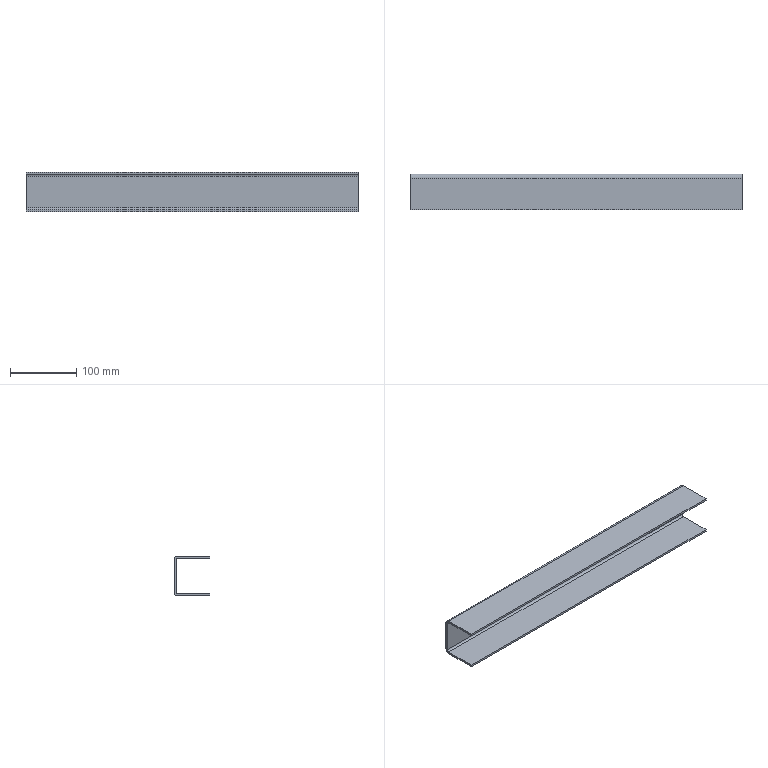Part | STEP file | JBJ-P-1015-02_Default<As Machined> | 1 solid | 22 faces | box 500 x 54 x 60 mm | volume 237206 mm3 | plane 18 | cylinder 4 | commonest cylinder face diameters 6 x2 12 x2
STEP:
#1=CARTESIAN_POINT('',(500.,54.,-6.));
#2=VERTEX_POINT('',#1);
#3=CARTESIAN_POINT('',(500.,51.,-6.));
#4=VERTEX_POINT('',#3);
#5=CARTESIAN_POINT('',(500.,54.,-6.));
#6=DIRECTION('',(0.,-1.,0.));
#7=VECTOR('',#6,1000.);
#8=LINE('',#5,#7);
#9=EDGE_CURVE('',#2,#4,#8,.T.);
#10=ORIENTED_EDGE('',*,*,#9,.F.);
#11=CARTESIAN_POINT('',(500.,48.,0.));
#12=VERTEX_POINT('',#11);
#13=CARTESIAN_POINT('',(500.,48.,-6.));
#14=DIRECTION('',(-1.,0.,0.));
#15=DIRECTION('',(0.,0.,-1.));
#16=AXIS2_PLACEMENT_3D('',#13,#14,#15);
#17=CIRCLE('',#16,6.);
#18=EDGE_CURVE('',#12,#2,#17,.T.);
#19=ORIENTED_EDGE('',*,*,#18,.F.);
#20=CARTESIAN_POINT('',(500.,48.,-3.));
#21=VERTEX_POINT('',#20);
#22=CARTESIAN_POINT('',(500.,48.,-3.));
#23=DIRECTION('',(0.,0.,1.));
#24=VECTOR('',#23,1000.);
#25=LINE('',#22,#24);
#26=EDGE_CURVE('',#21,#12,#25,.T.);
#27=ORIENTED_EDGE('',*,*,#26,.F.);
#28=CARTESIAN_POINT('',(500.,48.,-6.));
#29=DIRECTION('',(-1.,0.,0.));
#30=DIRECTION('',(0.,0.,-1.));
#31=AXIS2_PLACEMENT_3D('',#28,#29,#30);
#32=CIRCLE('',#31,3.);
#33=EDGE_CURVE('',#21,#4,#32,.T.);
#34=ORIENTED_EDGE('',*,*,#33,.T.);
#35=EDGE_LOOP('',(#10,#19,#27,#34));
#36=FACE_OUTER_BOUND('',#35,.T.);
#37=CARTESIAN_POINT('',(500.,54.,-6.));
#38=DIRECTION('',(1.,0.,0.));
#39=DIRECTION('',(0.,0.,-1.));
#40=AXIS2_PLACEMENT_3D('',#37,#38,#39);
#41=PLANE('',#40);
#42=ADVANCED_FACE('',(#36),#41,.T.);
#43=CARTESIAN_POINT('',(500.,54.,-54.));
#44=VERTEX_POINT('',#43);
#45=CARTESIAN_POINT('',(500.,54.,0.));
#46=DIRECTION('',(0.,0.,-1.));
#47=VECTOR('',#46,1000.);
#48=LINE('',#45,#47);
#49=EDGE_CURVE('',#2,#44,#48,.T.);
#50=ORIENTED_EDGE('',*,*,#49,.F.);
#51=ORIENTED_EDGE('',*,*,#9,.T.);
#52=CARTESIAN_POINT('',(500.,51.,-54.));
#53=VERTEX_POINT('',#52);
#54=CARTESIAN_POINT('',(500.,51.,0.));
#55=DIRECTION('',(0.,0.,-1.));
#56=VECTOR('',#55,1000.);
#57=LINE('',#54,#56);
#58=EDGE_CURVE('',#4,#53,#57,.T.);
#59=ORIENTED_EDGE('',*,*,#58,.T.);
#60=CARTESIAN_POINT('',(500.,51.,-54.));
#61=DIRECTION('',(0.,1.,0.));
#62=VECTOR('',#61,1000.);
#63=LINE('',#60,#62);
#64=EDGE_CURVE('',#53,#44,#63,.T.);
#65=ORIENTED_EDGE('',*,*,#64,.T.);
#66=EDGE_LOOP('',(#50,#51,#59,#65));
#67=FACE_OUTER_BOUND('',#66,.T.);
#68=CARTESIAN_POINT('',(500.,48.,-3.));
#69=DIRECTION('',(1.,0.,0.));
#70=DIRECTION('',(0.,0.,-1.));
#71=AXIS2_PLACEMENT_3D('',#68,#69,#70);
#72=PLANE('',#71);
#73=ADVANCED_FACE('',(#67),#72,.T.);
#74=CARTESIAN_POINT('',(0.,48.,0.));
#75=VERTEX_POINT('',#74);
#76=CARTESIAN_POINT('',(0.,48.,-3.));
#77=VERTEX_POINT('',#76);
#78=CARTESIAN_POINT('',(0.,48.,0.));
#79=DIRECTION('',(0.,0.,-1.));
#80=VECTOR('',#79,1000.);
#81=LINE('',#78,#80);
#82=EDGE_CURVE('',#75,#77,#81,.T.);
#83=ORIENTED_EDGE('',*,*,#82,.F.);
#84=CARTESIAN_POINT('',(0.,54.,-6.));
#85=VERTEX_POINT('',#84);
#86=CARTESIAN_POINT('',(0.,48.,-6.));
#87=DIRECTION('',(-1.,0.,0.));
#88=DIRECTION('',(0.,0.,-1.));
#89=AXIS2_PLACEMENT_3D('',#86,#87,#88);
#90=CIRCLE('',#89,6.);
#91=EDGE_CURVE('',#75,#85,#90,.T.);
#92=ORIENTED_EDGE('',*,*,#91,.T.);
#93=CARTESIAN_POINT('',(0.,51.,-6.));
#94=VERTEX_POINT('',#93);
#95=CARTESIAN_POINT('',(0.,51.,-6.));
#96=DIRECTION('',(0.,1.,0.));
#97=VECTOR('',#96,1000.);
#98=LINE('',#95,#97);
#99=EDGE_CURVE('',#94,#85,#98,.T.);
#100=ORIENTED_EDGE('',*,*,#99,.F.);
#101=CARTESIAN_POINT('',(0.,48.,-6.));
#102=DIRECTION('',(-1.,0.,0.));
#103=DIRECTION('',(0.,0.,-1.));
#104=AXIS2_PLACEMENT_3D('',#101,#102,#103);
#105=CIRCLE('',#104,3.);
#106=EDGE_CURVE('',#77,#94,#105,.T.);
#107=ORIENTED_EDGE('',*,*,#106,.F.);
#108=EDGE_LOOP('',(#83,#92,#100,#107));
#109=FACE_OUTER_BOUND('',#108,.T.);
#110=CARTESIAN_POINT('',(0.,48.,0.));
#111=DIRECTION('',(-1.,0.,0.));
#112=DIRECTION('',(0.,0.,1.));
#113=AXIS2_PLACEMENT_3D('',#110,#111,#112);
#114=PLANE('',#113);
#115=ADVANCED_FACE('',(#109),#114,.T.);
#116=CARTESIAN_POINT('',(0.,0.,0.));
#117=VERTEX_POINT('',#116);
#118=CARTESIAN_POINT('',(0.,0.,0.));
#119=DIRECTION('',(0.,1.,0.));
#120=VECTOR('',#119,1000.);
#121=LINE('',#118,#120);
#122=EDGE_CURVE('',#117,#75,#121,.T.);
#123=ORIENTED_EDGE('',*,*,#122,.T.);
#124=ORIENTED_EDGE('',*,*,#82,.T.);
#125=CARTESIAN_POINT('',(0.,0.,-3.));
#126=VERTEX_POINT('',#125);
#127=CARTESIAN_POINT('',(0.,0.,-3.));
#128=DIRECTION('',(0.,1.,0.));
#129=VECTOR('',#128,1000.);
#130=LINE('',#127,#129);
#131=EDGE_CURVE('',#126,#77,#130,.T.);
#132=ORIENTED_EDGE('',*,*,#131,.F.);
#133=CARTESIAN_POINT('',(0.,0.,-3.));
#134=DIRECTION('',(0.,0.,1.));
#135=VECTOR('',#134,1000.);
#136=LINE('',#133,#135);
#137=EDGE_CURVE('',#126,#117,#136,.T.);
#138=ORIENTED_EDGE('',*,*,#137,.T.);
#139=EDGE_LOOP('',(#123,#124,#132,#138));
#140=FACE_OUTER_BOUND('',#139,.T.);
#141=CARTESIAN_POINT('',(0.,51.,-6.));
#142=DIRECTION('',(-1.,0.,0.));
#143=DIRECTION('',(0.,0.,1.));
#144=AXIS2_PLACEMENT_3D('',#141,#142,#143);
#145=PLANE('',#144);
#146=ADVANCED_FACE('',(#140),#145,.T.);
#147=CARTESIAN_POINT('',(500.,48.,-60.));
#148=VERTEX_POINT('',#147);
#149=CARTESIAN_POINT('',(500.,48.,-57.));
#150=VERTEX_POINT('',#149);
#151=CARTESIAN_POINT('',(500.,48.,-60.));
#152=DIRECTION('',(0.,0.,1.));
#153=VECTOR('',#152,1000.);
#154=LINE('',#151,#153);
#155=EDGE_CURVE('',#148,#150,#154,.T.);
#156=ORIENTED_EDGE('',*,*,#155,.F.);
#157=CARTESIAN_POINT('',(500.,48.,-54.));
#158=DIRECTION('',(-1.,0.,0.));
#159=DIRECTION('',(0.,0.,-1.));
#160=AXIS2_PLACEMENT_3D('',#157,#158,#159);
#161=CIRCLE('',#160,6.);
#162=EDGE_CURVE('',#44,#148,#161,.T.);
#163=ORIENTED_EDGE('',*,*,#162,.F.);
#164=ORIENTED_EDGE('',*,*,#64,.F.);
#165=CARTESIAN_POINT('',(500.,48.,-54.));
#166=DIRECTION('',(-1.,0.,0.));
#167=DIRECTION('',(0.,0.,-1.));
#168=AXIS2_PLACEMENT_3D('',#165,#166,#167);
#169=CIRCLE('',#168,3.);
#170=EDGE_CURVE('',#53,#150,#169,.T.);
#171=ORIENTED_EDGE('',*,*,#170,.T.);
#172=EDGE_LOOP('',(#156,#163,#164,#171));
#173=FACE_OUTER_BOUND('',#172,.T.);
#174=CARTESIAN_POINT('',(500.,48.,-60.));
#175=DIRECTION('',(1.,0.,0.));
#176=DIRECTION('',(0.,0.,-1.));
#177=AXIS2_PLACEMENT_3D('',#174,#175,#176);
#178=PLANE('',#177);
#179=ADVANCED_FACE('',(#173),#178,.T.);
#180=CARTESIAN_POINT('',(500.,0.,-60.));
#181=VERTEX_POINT('',#180);
#182=CARTESIAN_POINT('',(500.,54.,-60.));
#183=DIRECTION('',(0.,-1.,0.));
#184=VECTOR('',#183,1000.);
#185=LINE('',#182,#184);
#186=EDGE_CURVE('',#148,#181,#185,.T.);
#187=ORIENTED_EDGE('',*,*,#186,.F.);
#188=ORIENTED_EDGE('',*,*,#155,.T.);
#189=CARTESIAN_POINT('',(500.,0.,-57.));
#190=VERTEX_POINT('',#189);
#191=CARTESIAN_POINT('',(500.,54.,-57.));
#192=DIRECTION('',(0.,-1.,0.));
#193=VECTOR('',#192,1000.);
#194=LINE('',#191,#193);
#195=EDGE_CURVE('',#150,#190,#194,.T.);
#196=ORIENTED_EDGE('',*,*,#195,.T.);
#197=CARTESIAN_POINT('',(500.,0.,-60.));
#198=DIRECTION('',(0.,0.,1.));
#199=VECTOR('',#198,1000.);
#200=LINE('',#197,#199);
#201=EDGE_CURVE('',#181,#190,#200,.T.);
#202=ORIENTED_EDGE('',*,*,#201,.F.);
#203=EDGE_LOOP('',(#187,#188,#196,#202));
#204=FACE_OUTER_BOUND('',#203,.T.);
#205=CARTESIAN_POINT('',(500.,51.,-54.));
#206=DIRECTION('',(1.,0.,0.));
#207=DIRECTION('',(0.,0.,-1.));
#208=AXIS2_PLACEMENT_3D('',#205,#206,#207);
#209=PLANE('',#208);
#210=ADVANCED_FACE('',(#204),#209,.T.);
#211=CARTESIAN_POINT('',(0.,54.,-54.));
#212=VERTEX_POINT('',#211);
#213=CARTESIAN_POINT('',(0.,51.,-54.));
#214=VERTEX_POINT('',#213);
#215=CARTESIAN_POINT('',(0.,54.,-54.));
#216=DIRECTION('',(0.,-1.,0.));
#217=VECTOR('',#216,1000.);
#218=LINE('',#215,#217);
#219=EDGE_CURVE('',#212,#214,#218,.T.);
#220=ORIENTED_EDGE('',*,*,#219,.F.);
#221=CARTESIAN_POINT('',(0.,48.,-60.));
#222=VERTEX_POINT('',#221);
#223=CARTESIAN_POINT('',(0.,48.,-54.));
#224=DIRECTION('',(-1.,0.,0.));
#225=DIRECTION('',(0.,0.,-1.));
#226=AXIS2_PLACEMENT_3D('',#223,#224,#225);
#227=CIRCLE('',#226,6.);
#228=EDGE_CURVE('',#212,#222,#227,.T.);
#229=ORIENTED_EDGE('',*,*,#228,.T.);
#230=CARTESIAN_POINT('',(0.,48.,-57.));
#231=VERTEX_POINT('',#230);
#232=CARTESIAN_POINT('',(0.,48.,-57.));
#233=DIRECTION('',(0.,0.,-1.));
#234=VECTOR('',#233,1000.);
#235=LINE('',#232,#234);
#236=EDGE_CURVE('',#231,#222,#235,.T.);
#237=ORIENTED_EDGE('',*,*,#236,.F.);
#238=CARTESIAN_POINT('',(0.,48.,-54.));
#239=DIRECTION('',(-1.,0.,0.));
#240=DIRECTION('',(0.,0.,-1.));
#241=AXIS2_PLACEMENT_3D('',#238,#239,#240);
#242=CIRCLE('',#241,3.);
#243=EDGE_CURVE('',#214,#231,#242,.T.);
#244=ORIENTED_EDGE('',*,*,#243,.F.);
#245=EDGE_LOOP('',(#220,#229,#237,#244));
#246=FACE_OUTER_BOUND('',#245,.T.);
#247=CARTESIAN_POINT('',(0.,54.,-54.));
#248=DIRECTION('',(-1.,0.,0.));
#249=DIRECTION('',(0.,0.,1.));
#250=AXIS2_PLACEMENT_3D('',#247,#248,#249);
#251=PLANE('',#250);
#252=ADVANCED_FACE('',(#246),#251,.T.);
#253=CARTESIAN_POINT('',(0.,54.,0.));
#254=DIRECTION('',(0.,0.,-1.));
#255=VECTOR('',#254,1000.);
#256=LINE('',#253,#255);
#257=EDGE_CURVE('',#85,#212,#256,.T.);
#258=ORIENTED_EDGE('',*,*,#257,.T.);
#259=ORIENTED_EDGE('',*,*,#219,.T.);
#260=CARTESIAN_POINT('',(0.,51.,0.));
#261=DIRECTION('',(0.,0.,-1.));
#262=VECTOR('',#261,1000.);
#263=LINE('',#260,#262);
#264=EDGE_CURVE('',#94,#214,#263,.T.);
#265=ORIENTED_EDGE('',*,*,#264,.F.);
#266=ORIENTED_EDGE('',*,*,#99,.T.);
#267=EDGE_LOOP('',(#258,#259,#265,#266));
#268=FACE_OUTER_BOUND('',#267,.T.);
#269=CARTESIAN_POINT('',(0.,48.,-57.));
#270=DIRECTION('',(-1.,0.,0.));
#271=DIRECTION('',(0.,0.,1.));
#272=AXIS2_PLACEMENT_3D('',#269,#270,#271);
#273=PLANE('',#272);
#274=ADVANCED_FACE('',(#268),#273,.T.);
#275=CARTESIAN_POINT('',(0.,0.,-57.));
#276=VERTEX_POINT('',#275);
#277=CARTESIAN_POINT('',(0.,54.,-57.));
#278=DIRECTION('',(0.,-1.,0.));
#279=VECTOR('',#278,1000.);
#280=LINE('',#277,#279);
#281=EDGE_CURVE('',#231,#276,#280,.T.);
#282=ORIENTED_EDGE('',*,*,#281,.T.);
#283=CARTESIAN_POINT('',(500.,0.,-57.));
#284=DIRECTION('',(-1.,0.,0.));
#285=VECTOR('',#284,1000.);
#286=LINE('',#283,#285);
#287=EDGE_CURVE('',#190,#276,#286,.T.);
#288=ORIENTED_EDGE('',*,*,#287,.F.);
#289=ORIENTED_EDGE('',*,*,#195,.F.);
#290=CARTESIAN_POINT('',(500.,48.,-57.));
#291=DIRECTION('',(-1.,0.,0.));
#292=VECTOR('',#291,1000.);
#293=LINE('',#290,#292);
#294=EDGE_CURVE('',#150,#231,#293,.T.);
#295=ORIENTED_EDGE('',*,*,#294,.T.);
#296=EDGE_LOOP('',(#282,#288,#289,#295));
#297=FACE_OUTER_BOUND('',#296,.T.);
#298=CARTESIAN_POINT('',(500.,54.,-57.));
#299=DIRECTION('',(0.,0.,-1.));
#300=DIRECTION('',(-1.,0.,0.));
#301=AXIS2_PLACEMENT_3D('',#298,#299,#300);
#302=PLANE('',#301);
#303=ADVANCED_FACE('',(#297),#302,.F.);
#304=CARTESIAN_POINT('',(0.,0.,-60.));
#305=VERTEX_POINT('',#304);
#306=CARTESIAN_POINT('',(0.,0.,-60.));
#307=DIRECTION('',(0.,0.,1.));
#308=VECTOR('',#307,1000.);
#309=LINE('',#306,#308);
#310=EDGE_CURVE('',#305,#276,#309,.T.);
#311=ORIENTED_EDGE('',*,*,#310,.F.);
#312=CARTESIAN_POINT('',(500.,0.,-60.));
#313=DIRECTION('',(-1.,0.,0.));
#314=VECTOR('',#313,1000.);
#315=LINE('',#312,#314);
#316=EDGE_CURVE('',#181,#305,#315,.T.);
#317=ORIENTED_EDGE('',*,*,#316,.F.);
#318=ORIENTED_EDGE('',*,*,#201,.T.);
#319=ORIENTED_EDGE('',*,*,#287,.T.);
#320=EDGE_LOOP('',(#311,#317,#318,#319));
#321=FACE_OUTER_BOUND('',#320,.T.);
#322=CARTESIAN_POINT('',(500.,0.,-60.));
#323=DIRECTION('',(0.,-1.,0.));
#324=DIRECTION('',(0.,0.,-1.));
#325=AXIS2_PLACEMENT_3D('',#322,#323,#324);
#326=PLANE('',#325);
#327=ADVANCED_FACE('',(#321),#326,.T.);
#328=CARTESIAN_POINT('',(0.,54.,-60.));
#329=DIRECTION('',(0.,-1.,0.));
#330=VECTOR('',#329,1000.);
#331=LINE('',#328,#330);
#332=EDGE_CURVE('',#222,#305,#331,.T.);
#333=ORIENTED_EDGE('',*,*,#332,.F.);
#334=CARTESIAN_POINT('',(500.,48.,-60.));
#335=DIRECTION('',(-1.,0.,0.));
#336=VECTOR('',#335,1000.);
#337=LINE('',#334,#336);
#338=EDGE_CURVE('',#148,#222,#337,.T.);
#339=ORIENTED_EDGE('',*,*,#338,.F.);
#340=ORIENTED_EDGE('',*,*,#186,.T.);
#341=ORIENTED_EDGE('',*,*,#316,.T.);
#342=EDGE_LOOP('',(#333,#339,#340,#341));
#343=FACE_OUTER_BOUND('',#342,.T.);
#344=CARTESIAN_POINT('',(500.,54.,-60.));
#345=DIRECTION('',(0.,0.,-1.));
#346=DIRECTION('',(-1.,0.,0.));
#347=AXIS2_PLACEMENT_3D('',#344,#345,#346);
#348=PLANE('',#347);
#349=ADVANCED_FACE('',(#343),#348,.T.);
#350=ORIENTED_EDGE('',*,*,#228,.F.);
#351=CARTESIAN_POINT('',(500.,54.,-54.));
#352=DIRECTION('',(-1.,0.,0.));
#353=VECTOR('',#352,1000.);
#354=LINE('',#351,#353);
#355=EDGE_CURVE('',#44,#212,#354,.T.);
#356=ORIENTED_EDGE('',*,*,#355,.F.);
#357=ORIENTED_EDGE('',*,*,#162,.T.);
#358=ORIENTED_EDGE('',*,*,#338,.T.);
#359=EDGE_LOOP('',(#350,#356,#357,#358));
#360=FACE_OUTER_BOUND('',#359,.T.);
#361=CARTESIAN_POINT('',(500.,48.,-54.));
#362=DIRECTION('',(-1.,0.,0.));
#363=DIRECTION('',(0.,0.,1.));
#364=AXIS2_PLACEMENT_3D('',#361,#362,#363);
#365=CYLINDRICAL_SURFACE('',#364,6.);
#366=ADVANCED_FACE('',(#360),#365,.T.);
#367=ORIENTED_EDGE('',*,*,#257,.F.);
#368=CARTESIAN_POINT('',(500.,54.,-6.));
#369=DIRECTION('',(-1.,0.,0.));
#370=VECTOR('',#369,1000.);
#371=LINE('',#368,#370);
#372=EDGE_CURVE('',#2,#85,#371,.T.);
#373=ORIENTED_EDGE('',*,*,#372,.F.);
#374=ORIENTED_EDGE('',*,*,#49,.T.);
#375=ORIENTED_EDGE('',*,*,#355,.T.);
#376=EDGE_LOOP('',(#367,#373,#374,#375));
#377=FACE_OUTER_BOUND('',#376,.T.);
#378=CARTESIAN_POINT('',(500.,54.,0.));
#379=DIRECTION('',(0.,1.,0.));
#380=DIRECTION('',(0.,0.,1.));
#381=AXIS2_PLACEMENT_3D('',#378,#379,#380);
#382=PLANE('',#381);
#383=ADVANCED_FACE('',(#377),#382,.T.);
#384=ORIENTED_EDGE('',*,*,#91,.F.);
#385=CARTESIAN_POINT('',(500.,48.,0.));
#386=DIRECTION('',(-1.,0.,0.));
#387=VECTOR('',#386,1000.);
#388=LINE('',#385,#387);
#389=EDGE_CURVE('',#12,#75,#388,.T.);
#390=ORIENTED_EDGE('',*,*,#389,.F.);
#391=ORIENTED_EDGE('',*,*,#18,.T.);
#392=ORIENTED_EDGE('',*,*,#372,.T.);
#393=EDGE_LOOP('',(#384,#390,#391,#392));
#394=FACE_OUTER_BOUND('',#393,.T.);
#395=CARTESIAN_POINT('',(500.,48.,-6.));
#396=DIRECTION('',(-1.,0.,0.));
#397=DIRECTION('',(0.,0.,1.));
#398=AXIS2_PLACEMENT_3D('',#395,#396,#397);
#399=CYLINDRICAL_SURFACE('',#398,6.);
#400=ADVANCED_FACE('',(#394),#399,.T.);
#401=ORIENTED_EDGE('',*,*,#122,.F.);
#402=CARTESIAN_POINT('',(500.,0.,0.));
#403=VERTEX_POINT('',#402);
#404=CARTESIAN_POINT('',(500.,0.,0.));
#405=DIRECTION('',(-1.,0.,0.));
#406=VECTOR('',#405,1000.);
#407=LINE('',#404,#406);
#408=EDGE_CURVE('',#403,#117,#407,.T.);
#409=ORIENTED_EDGE('',*,*,#408,.F.);
#410=CARTESIAN_POINT('',(500.,0.,0.));
#411=DIRECTION('',(0.,1.,0.));
#412=VECTOR('',#411,1000.);
#413=LINE('',#410,#412);
#414=EDGE_CURVE('',#403,#12,#413,.T.);
#415=ORIENTED_EDGE('',*,*,#414,.T.);
#416=ORIENTED_EDGE('',*,*,#389,.T.);
#417=EDGE_LOOP('',(#401,#409,#415,#416));
#418=FACE_OUTER_BOUND('',#417,.T.);
#419=CARTESIAN_POINT('',(500.,0.,0.));
#420=DIRECTION('',(0.,0.,1.));
#421=DIRECTION('',(1.,0.,0.));
#422=AXIS2_PLACEMENT_3D('',#419,#420,#421);
#423=PLANE('',#422);
#424=ADVANCED_FACE('',(#418),#423,.T.);
#425=ORIENTED_EDGE('',*,*,#137,.F.);
#426=CARTESIAN_POINT('',(500.,0.,-3.));
#427=VERTEX_POINT('',#426);
#428=CARTESIAN_POINT('',(500.,0.,-3.));
#429=DIRECTION('',(-1.,0.,0.));
#430=VECTOR('',#429,1000.);
#431=LINE('',#428,#430);
#432=EDGE_CURVE('',#427,#126,#431,.T.);
#433=ORIENTED_EDGE('',*,*,#432,.F.);
#434=CARTESIAN_POINT('',(500.,0.,-3.));
#435=DIRECTION('',(0.,0.,1.));
#436=VECTOR('',#435,1000.);
#437=LINE('',#434,#436);
#438=EDGE_CURVE('',#427,#403,#437,.T.);
#439=ORIENTED_EDGE('',*,*,#438,.T.);
#440=ORIENTED_EDGE('',*,*,#408,.T.);
#441=EDGE_LOOP('',(#425,#433,#439,#440));
#442=FACE_OUTER_BOUND('',#441,.T.);
#443=CARTESIAN_POINT('',(500.,0.,-3.));
#444=DIRECTION('',(0.,-1.,0.));
#445=DIRECTION('',(0.,0.,-1.));
#446=AXIS2_PLACEMENT_3D('',#443,#444,#445);
#447=PLANE('',#446);
#448=ADVANCED_FACE('',(#442),#447,.T.);
#449=ORIENTED_EDGE('',*,*,#131,.T.);
#450=CARTESIAN_POINT('',(500.,48.,-3.));
#451=DIRECTION('',(-1.,0.,0.));
#452=VECTOR('',#451,1000.);
#453=LINE('',#450,#452);
#454=EDGE_CURVE('',#21,#77,#453,.T.);
#455=ORIENTED_EDGE('',*,*,#454,.F.);
#456=CARTESIAN_POINT('',(500.,0.,-3.));
#457=DIRECTION('',(0.,1.,0.));
#458=VECTOR('',#457,1000.);
#459=LINE('',#456,#458);
#460=EDGE_CURVE('',#427,#21,#459,.T.);
#461=ORIENTED_EDGE('',*,*,#460,.F.);
#462=ORIENTED_EDGE('',*,*,#432,.T.);
#463=EDGE_LOOP('',(#449,#455,#461,#462));
#464=FACE_OUTER_BOUND('',#463,.T.);
#465=CARTESIAN_POINT('',(500.,0.,-3.));
#466=DIRECTION('',(0.,0.,1.));
#467=DIRECTION('',(1.,0.,0.));
#468=AXIS2_PLACEMENT_3D('',#465,#466,#467);
#469=PLANE('',#468);
#470=ADVANCED_FACE('',(#464),#469,.F.);
#471=ORIENTED_EDGE('',*,*,#106,.T.);
#472=CARTESIAN_POINT('',(500.,51.,-6.));
#473=DIRECTION('',(-1.,0.,0.));
#474=VECTOR('',#473,1000.);
#475=LINE('',#472,#474);
#476=EDGE_CURVE('',#4,#94,#475,.T.);
#477=ORIENTED_EDGE('',*,*,#476,.F.);
#478=ORIENTED_EDGE('',*,*,#33,.F.);
#479=ORIENTED_EDGE('',*,*,#454,.T.);
#480=EDGE_LOOP('',(#471,#477,#478,#479));
#481=FACE_OUTER_BOUND('',#480,.T.);
#482=CARTESIAN_POINT('',(500.,48.,-6.));
#483=DIRECTION('',(-1.,0.,0.));
#484=DIRECTION('',(0.,0.,1.));
#485=AXIS2_PLACEMENT_3D('',#482,#483,#484);
#486=CYLINDRICAL_SURFACE('',#485,3.);
#487=ADVANCED_FACE('',(#481),#486,.F.);
#488=ORIENTED_EDGE('',*,*,#264,.T.);
#489=CARTESIAN_POINT('',(500.,51.,-54.));
#490=DIRECTION('',(-1.,0.,0.));
#491=VECTOR('',#490,1000.);
#492=LINE('',#489,#491);
#493=EDGE_CURVE('',#53,#214,#492,.T.);
#494=ORIENTED_EDGE('',*,*,#493,.F.);
#495=ORIENTED_EDGE('',*,*,#58,.F.);
#496=ORIENTED_EDGE('',*,*,#476,.T.);
#497=EDGE_LOOP('',(#488,#494,#495,#496));
#498=FACE_OUTER_BOUND('',#497,.T.);
#499=CARTESIAN_POINT('',(500.,51.,0.));
#500=DIRECTION('',(0.,1.,0.));
#501=DIRECTION('',(0.,0.,1.));
#502=AXIS2_PLACEMENT_3D('',#499,#500,#501);
#503=PLANE('',#502);
#504=ADVANCED_FACE('',(#498),#503,.F.);
#505=ORIENTED_EDGE('',*,*,#243,.T.);
#506=ORIENTED_EDGE('',*,*,#294,.F.);
#507=ORIENTED_EDGE('',*,*,#170,.F.);
#508=ORIENTED_EDGE('',*,*,#493,.T.);
#509=EDGE_LOOP('',(#505,#506,#507,#508));
#510=FACE_OUTER_BOUND('',#509,.T.);
#511=CARTESIAN_POINT('',(500.,48.,-54.));
#512=DIRECTION('',(-1.,0.,0.));
#513=DIRECTION('',(0.,0.,1.));
#514=AXIS2_PLACEMENT_3D('',#511,#512,#513);
#515=CYLINDRICAL_SURFACE('',#514,3.);
#516=ADVANCED_FACE('',(#510),#515,.F.);
#517=ORIENTED_EDGE('',*,*,#460,.T.);
#518=ORIENTED_EDGE('',*,*,#26,.T.);
#519=ORIENTED_EDGE('',*,*,#414,.F.);
#520=ORIENTED_EDGE('',*,*,#438,.F.);
#521=EDGE_LOOP('',(#517,#518,#519,#520));
#522=FACE_OUTER_BOUND('',#521,.T.);
#523=CARTESIAN_POINT('',(500.,48.,-54.));
#524=DIRECTION('',(1.,0.,0.));
#525=DIRECTION('',(0.,0.,-1.));
#526=AXIS2_PLACEMENT_3D('',#523,#524,#525);
#527=PLANE('',#526);
#528=ADVANCED_FACE('',(#522),#527,.T.);
#529=ORIENTED_EDGE('',*,*,#281,.F.);
#530=ORIENTED_EDGE('',*,*,#236,.T.);
#531=ORIENTED_EDGE('',*,*,#332,.T.);
#532=ORIENTED_EDGE('',*,*,#310,.T.);
#533=EDGE_LOOP('',(#529,#530,#531,#532));
#534=FACE_OUTER_BOUND('',#533,.T.);
#535=CARTESIAN_POINT('',(0.,48.,-54.));
#536=DIRECTION('',(1.,0.,0.));
#537=DIRECTION('',(0.,0.,-1.));
#538=AXIS2_PLACEMENT_3D('',#535,#536,#537);
#539=PLANE('',#538);
#540=ADVANCED_FACE('',(#534),#539,.F.);
#541=CLOSED_SHELL('',(#42,#73,#115,#146,#179,#210,#252,#274,#303,#327,#349,#366,#383,#400,#424,#448,#470,#487,#504,#516,#528,#540));
#542=MANIFOLD_SOLID_BREP('',#541);
#543=CARTESIAN_POINT('',(0.,0.,0.));
#544=DIRECTION('',(0.,0.,1.));
#545=DIRECTION('',(1.,0.,0.));
#546=AXIS2_PLACEMENT_3D('',#543,#544,#545);
#547=(LENGTH_UNIT()NAMED_UNIT(*)SI_UNIT(.MILLI.,.METRE.));
#548=UNCERTAINTY_MEASURE_WITH_UNIT(LENGTH_MEASURE(0.00001),#547,'','');
#549=(NAMED_UNIT(*)PLANE_ANGLE_UNIT()SI_UNIT($,.RADIAN.));
#550=(NAMED_UNIT(*)SI_UNIT($,.STERADIAN.)SOLID_ANGLE_UNIT());
#551=(GEOMETRIC_REPRESENTATION_CONTEXT(3)GLOBAL_UNCERTAINTY_ASSIGNED_CONTEXT((#548))GLOBAL_UNIT_ASSIGNED_CONTEXT((#547,#549,#550))REPRESENTATION_CONTEXT('',''));
#552=ADVANCED_BREP_SHAPE_REPRESENTATION('',(#542,#546),#551);